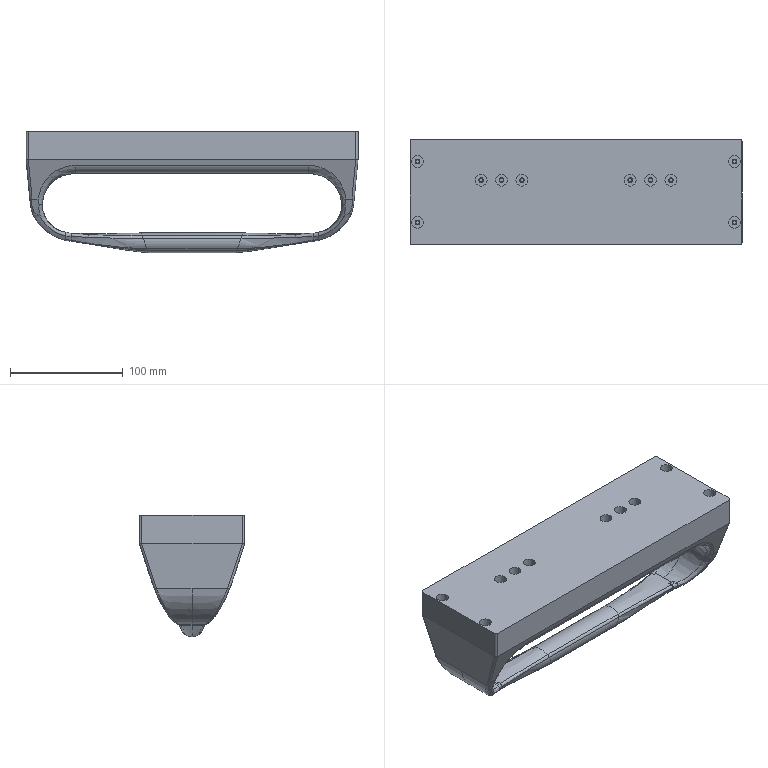NC program | NX | posted with a generic post | part box 294.078 x 93.5 x 107.5 mm
Lines 3664 to 3753 of 3753:
(ZLEVEL_PROFILE_1_COPY_1_COPY_COPY_1 , TOOL : D6A45)
N7290 T07 M6
N7292 G54
N7294 G17 G0 G90 X-131.533 Y-33.816 B0. C0. S7500 M3
N7296 G43 Z28.5 H7
N7298 Z-1.5
N7300 G94 G1 Z-2.5 F1000.
N7302 X-130.914 Y-34.888
N7304 G3 X-130.394 Y-35.188 R0.6
N7306 G1 X130.394
N7308 G3 X135.435 Y-30.147 R5.041
N7310 G1 Y-27.003
N7312 G2 X139.337 Y-22.156 R4.96
N7314 G3 X143.435 Y-17.19 R5.07
N7316 G1 Y17.179
N7318 G3 X139.337 Y22.156 R5.07
N7320 G2 X135.435 Y27.001 R4.959
N7322 G1 Y30.147
N7324 G3 X130.394 Y35.188 R5.041
N7326 G1 X-130.394
N7328 G3 X-135.435 Y30.147 R5.041
N7330 G1 Y27.003
N7332 G2 X-139.337 Y22.156 R4.961
N7334 G3 X-143.435 Y17.183 R5.071
N7336 G1 Y-17.182
N7338 G3 X-139.337 Y-22.156 R5.078
N7340 G2 X-135.435 Y-27.001 R4.96
N7342 G1 Y-30.147
N7344 G3 X-130.394 Y-35.188 R5.041
N7346 X-129.874 Y-34.888 R0.6
N7348 G1 X-129.355 Y-33.988
N7350 Z-1.5
N7352 G0 Z28.5
N7354 X-88.163 Y24.151
N7356 Z-1.5
N7358 G1 Z-2.5
N7360 X-87.686 Y23.325
N7362 G3 X-87.167 Y23.025 R0.6
N7364 G1 X-46.167
N7366 G2 X-40.708 Y17.567 R5.459
N7368 G1 Y3.
N7370 G2 X-46.167 Y-2.459 R5.459
N7372 G1 X-87.167
N7374 G2 X-92.625 Y3. R5.459
N7376 G1 Y17.567
N7378 G2 X-87.167 Y23.025 R5.459
N7380 G3 X-86.647 Y23.325 R0.6
N7382 G1 X-86.128 Y24.225
N7384 Z-1.5
N7386 G0 Z28.5
N7388 X45.254 Y24.151
N7390 Z-1.5
N7392 G1 Z-2.5
N7394 X45.73 Y23.325
N7396 G3 X46.25 Y23.025 R0.6
N7398 G1 X87.25
N7400 G2 X92.709 Y17.567 R5.459
N7402 G1 Y3.
N7404 G2 X87.25 Y-2.459 R5.459
N7406 G1 X46.25
N7408 G2 X40.791 Y3. R5.459
N7410 G1 Y17.567
N7412 G2 X46.25 Y23.025 R5.459
N7414 G3 X46.77 Y23.325 R0.6
N7416 G1 X47.289 Y24.225
N7418 Z-1.5
N7420 G0 Z28.5
N7422 X-146.033 Y48.789
N7424 Z-1.5
N7426 G1 Z-2.5
N7428 X-145.582 Y48.009
N7430 G3 X-145.063 Y47.709 R0.6
N7432 G1 X144.956
N7434 G2 X147.998 Y44.678 R3.009
N7436 G1 Y-44.647
N7438 G2 X145.032 Y-47.709 R3.014
N7440 G1 X-145.032
N7442 G2 X-147.759 Y-45.851 R2.964
N7444 X-147.998 Y-44.647 R3.249
N7446 G1 Y44.647
N7448 G2 X-146.468 Y47.328 R3.085
N7450 X-145.063 Y47.709 R2.788
N7452 G3 X-144.543 Y48.009 R0.6
N7454 G1 X-144.023 Y48.909
N7456 Z-1.5
N7458 G0 Z28.5
N7460 M5
N7462 M2